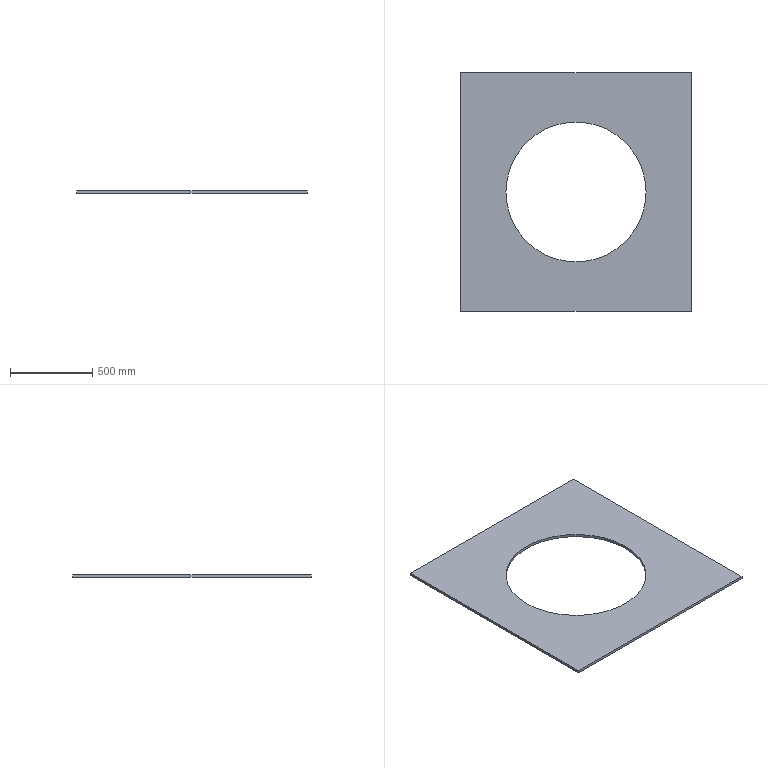Part | SolidWorks | features FlatPattern 1, ICE 1, SMBaseFlange 1, SheetMetal 1 | 1 solid | 8 faces | box 1400 x 1450 x 16 mm | volume 23400797 mm3 | plane 6 | cylinder 2 | commonest cylinder face diameters 850 x2
STEP:
#1=CARTESIAN_POINT('',(-425.,0.,-16.));
#2=VERTEX_POINT('',#1);
#3=CARTESIAN_POINT('',(425.,0.,-16.));
#4=VERTEX_POINT('',#3);
#5=CARTESIAN_POINT('',(0.,0.,-16.));
#6=DIRECTION('',(0.,0.,1.));
#7=DIRECTION('',(1.,0.,0.));
#8=AXIS2_PLACEMENT_3D('',#5,#6,#7);
#9=CIRCLE('',#8,425.);
#10=EDGE_CURVE('',#2,#4,#9,.T.);
#11=ORIENTED_EDGE('',*,*,#10,.F.);
#12=CARTESIAN_POINT('',(-425.,0.,0.));
#13=VERTEX_POINT('',#12);
#14=CARTESIAN_POINT('',(-425.,0.,-16.));
#15=DIRECTION('',(0.,0.,1.));
#16=VECTOR('',#15,1000.);
#17=LINE('',#14,#16);
#18=EDGE_CURVE('',#2,#13,#17,.T.);
#19=ORIENTED_EDGE('',*,*,#18,.T.);
#20=CARTESIAN_POINT('',(425.,0.,0.));
#21=VERTEX_POINT('',#20);
#22=CARTESIAN_POINT('',(0.,0.,0.));
#23=DIRECTION('',(0.,0.,1.));
#24=DIRECTION('',(1.,0.,0.));
#25=AXIS2_PLACEMENT_3D('',#22,#23,#24);
#26=CIRCLE('',#25,425.);
#27=EDGE_CURVE('',#13,#21,#26,.T.);
#28=ORIENTED_EDGE('',*,*,#27,.T.);
#29=CARTESIAN_POINT('',(425.,0.,-16.));
#30=DIRECTION('',(0.,0.,1.));
#31=VECTOR('',#30,1000.);
#32=LINE('',#29,#31);
#33=EDGE_CURVE('',#4,#21,#32,.T.);
#34=ORIENTED_EDGE('',*,*,#33,.F.);
#35=EDGE_LOOP('',(#11,#19,#28,#34));
#36=FACE_OUTER_BOUND('',#35,.T.);
#37=CARTESIAN_POINT('',(0.,0.,-16.));
#38=DIRECTION('',(0.,0.,1.));
#39=DIRECTION('',(1.,0.,0.));
#40=AXIS2_PLACEMENT_3D('',#37,#38,#39);
#41=CYLINDRICAL_SURFACE('',#40,425.);
#42=ADVANCED_FACE('',(#36),#41,.F.);
#43=CARTESIAN_POINT('',(700.,-725.,0.));
#44=VERTEX_POINT('',#43);
#45=CARTESIAN_POINT('',(700.,725.,0.));
#46=VERTEX_POINT('',#45);
#47=CARTESIAN_POINT('',(700.,-725.,0.));
#48=DIRECTION('',(0.,1.,0.));
#49=VECTOR('',#48,1000.);
#50=LINE('',#47,#49);
#51=EDGE_CURVE('',#44,#46,#50,.T.);
#52=ORIENTED_EDGE('',*,*,#51,.F.);
#53=CARTESIAN_POINT('',(700.,-725.,-16.));
#54=VERTEX_POINT('',#53);
#55=CARTESIAN_POINT('',(700.,-725.,-16.));
#56=DIRECTION('',(0.,0.,1.));
#57=VECTOR('',#56,1000.);
#58=LINE('',#55,#57);
#59=EDGE_CURVE('',#54,#44,#58,.T.);
#60=ORIENTED_EDGE('',*,*,#59,.F.);
#61=CARTESIAN_POINT('',(700.,725.,-16.));
#62=VERTEX_POINT('',#61);
#63=CARTESIAN_POINT('',(700.,-725.,-16.));
#64=DIRECTION('',(0.,1.,0.));
#65=VECTOR('',#64,1000.);
#66=LINE('',#63,#65);
#67=EDGE_CURVE('',#54,#62,#66,.T.);
#68=ORIENTED_EDGE('',*,*,#67,.T.);
#69=CARTESIAN_POINT('',(700.,725.,-16.));
#70=DIRECTION('',(0.,0.,1.));
#71=VECTOR('',#70,1000.);
#72=LINE('',#69,#71);
#73=EDGE_CURVE('',#62,#46,#72,.T.);
#74=ORIENTED_EDGE('',*,*,#73,.T.);
#75=EDGE_LOOP('',(#52,#60,#68,#74));
#76=FACE_OUTER_BOUND('',#75,.T.);
#77=CARTESIAN_POINT('',(700.,-725.,-16.));
#78=DIRECTION('',(1.,0.,0.));
#79=DIRECTION('',(0.,0.,-1.));
#80=AXIS2_PLACEMENT_3D('',#77,#78,#79);
#81=PLANE('',#80);
#82=ADVANCED_FACE('',(#76),#81,.T.);
#83=CARTESIAN_POINT('',(-700.,-725.,0.));
#84=VERTEX_POINT('',#83);
#85=CARTESIAN_POINT('',(-700.,-725.,0.));
#86=DIRECTION('',(1.,0.,0.));
#87=VECTOR('',#86,1000.);
#88=LINE('',#85,#87);
#89=EDGE_CURVE('',#84,#44,#88,.T.);
#90=ORIENTED_EDGE('',*,*,#89,.F.);
#91=CARTESIAN_POINT('',(-700.,-725.,-16.));
#92=VERTEX_POINT('',#91);
#93=CARTESIAN_POINT('',(-700.,-725.,-16.));
#94=DIRECTION('',(0.,0.,1.));
#95=VECTOR('',#94,1000.);
#96=LINE('',#93,#95);
#97=EDGE_CURVE('',#92,#84,#96,.T.);
#98=ORIENTED_EDGE('',*,*,#97,.F.);
#99=CARTESIAN_POINT('',(-700.,-725.,-16.));
#100=DIRECTION('',(1.,0.,0.));
#101=VECTOR('',#100,1000.);
#102=LINE('',#99,#101);
#103=EDGE_CURVE('',#92,#54,#102,.T.);
#104=ORIENTED_EDGE('',*,*,#103,.T.);
#105=ORIENTED_EDGE('',*,*,#59,.T.);
#106=EDGE_LOOP('',(#90,#98,#104,#105));
#107=FACE_OUTER_BOUND('',#106,.T.);
#108=CARTESIAN_POINT('',(-700.,-725.,-16.));
#109=DIRECTION('',(0.,-1.,0.));
#110=DIRECTION('',(0.,0.,-1.));
#111=AXIS2_PLACEMENT_3D('',#108,#109,#110);
#112=PLANE('',#111);
#113=ADVANCED_FACE('',(#107),#112,.T.);
#114=CARTESIAN_POINT('',(-700.,725.,0.));
#115=VERTEX_POINT('',#114);
#116=CARTESIAN_POINT('',(-700.,-725.,0.));
#117=DIRECTION('',(0.,-1.,0.));
#118=VECTOR('',#117,1000.);
#119=LINE('',#116,#118);
#120=EDGE_CURVE('',#115,#84,#119,.T.);
#121=ORIENTED_EDGE('',*,*,#120,.F.);
#122=CARTESIAN_POINT('',(-700.,725.,-16.));
#123=VERTEX_POINT('',#122);
#124=CARTESIAN_POINT('',(-700.,725.,-16.));
#125=DIRECTION('',(0.,0.,1.));
#126=VECTOR('',#125,1000.);
#127=LINE('',#124,#126);
#128=EDGE_CURVE('',#123,#115,#127,.T.);
#129=ORIENTED_EDGE('',*,*,#128,.F.);
#130=CARTESIAN_POINT('',(-700.,-725.,-16.));
#131=DIRECTION('',(0.,-1.,0.));
#132=VECTOR('',#131,1000.);
#133=LINE('',#130,#132);
#134=EDGE_CURVE('',#123,#92,#133,.T.);
#135=ORIENTED_EDGE('',*,*,#134,.T.);
#136=ORIENTED_EDGE('',*,*,#97,.T.);
#137=EDGE_LOOP('',(#121,#129,#135,#136));
#138=FACE_OUTER_BOUND('',#137,.T.);
#139=CARTESIAN_POINT('',(-700.,-725.,-16.));
#140=DIRECTION('',(-1.,0.,0.));
#141=DIRECTION('',(0.,0.,1.));
#142=AXIS2_PLACEMENT_3D('',#139,#140,#141);
#143=PLANE('',#142);
#144=ADVANCED_FACE('',(#138),#143,.T.);
#145=CARTESIAN_POINT('',(-700.,725.,0.));
#146=DIRECTION('',(-1.,0.,0.));
#147=VECTOR('',#146,1000.);
#148=LINE('',#145,#147);
#149=EDGE_CURVE('',#46,#115,#148,.T.);
#150=ORIENTED_EDGE('',*,*,#149,.F.);
#151=ORIENTED_EDGE('',*,*,#73,.F.);
#152=CARTESIAN_POINT('',(-700.,725.,-16.));
#153=DIRECTION('',(-1.,0.,0.));
#154=VECTOR('',#153,1000.);
#155=LINE('',#152,#154);
#156=EDGE_CURVE('',#62,#123,#155,.T.);
#157=ORIENTED_EDGE('',*,*,#156,.T.);
#158=ORIENTED_EDGE('',*,*,#128,.T.);
#159=EDGE_LOOP('',(#150,#151,#157,#158));
#160=FACE_OUTER_BOUND('',#159,.T.);
#161=CARTESIAN_POINT('',(-700.,725.,-16.));
#162=DIRECTION('',(0.,1.,0.));
#163=DIRECTION('',(0.,0.,1.));
#164=AXIS2_PLACEMENT_3D('',#161,#162,#163);
#165=PLANE('',#164);
#166=ADVANCED_FACE('',(#160),#165,.T.);
#167=CARTESIAN_POINT('',(0.,0.,-16.));
#168=DIRECTION('',(0.,0.,1.));
#169=DIRECTION('',(1.,0.,0.));
#170=AXIS2_PLACEMENT_3D('',#167,#168,#169);
#171=CIRCLE('',#170,425.);
#172=EDGE_CURVE('',#4,#2,#171,.T.);
#173=ORIENTED_EDGE('',*,*,#172,.T.);
#174=ORIENTED_EDGE('',*,*,#10,.T.);
#175=EDGE_LOOP('',(#173,#174));
#176=FACE_BOUND('',#175,.T.);
#177=ORIENTED_EDGE('',*,*,#67,.F.);
#178=ORIENTED_EDGE('',*,*,#103,.F.);
#179=ORIENTED_EDGE('',*,*,#134,.F.);
#180=ORIENTED_EDGE('',*,*,#156,.F.);
#181=EDGE_LOOP('',(#177,#178,#179,#180));
#182=FACE_OUTER_BOUND('',#181,.T.);
#183=CARTESIAN_POINT('',(0.,0.,-16.));
#184=DIRECTION('',(0.,0.,-1.));
#185=DIRECTION('',(-1.,0.,0.));
#186=AXIS2_PLACEMENT_3D('',#183,#184,#185);
#187=PLANE('',#186);
#188=ADVANCED_FACE('',(#176,#182),#187,.T.);
#189=CARTESIAN_POINT('',(0.,0.,0.));
#190=DIRECTION('',(0.,0.,1.));
#191=DIRECTION('',(1.,0.,0.));
#192=AXIS2_PLACEMENT_3D('',#189,#190,#191);
#193=CIRCLE('',#192,425.);
#194=EDGE_CURVE('',#21,#13,#193,.T.);
#195=ORIENTED_EDGE('',*,*,#194,.F.);
#196=ORIENTED_EDGE('',*,*,#27,.F.);
#197=EDGE_LOOP('',(#195,#196));
#198=FACE_BOUND('',#197,.T.);
#199=ORIENTED_EDGE('',*,*,#51,.T.);
#200=ORIENTED_EDGE('',*,*,#149,.T.);
#201=ORIENTED_EDGE('',*,*,#120,.T.);
#202=ORIENTED_EDGE('',*,*,#89,.T.);
#203=EDGE_LOOP('',(#199,#200,#201,#202));
#204=FACE_OUTER_BOUND('',#203,.T.);
#205=CARTESIAN_POINT('',(0.,0.,0.));
#206=DIRECTION('',(0.,0.,-1.));
#207=DIRECTION('',(-1.,0.,0.));
#208=AXIS2_PLACEMENT_3D('',#205,#206,#207);
#209=PLANE('',#208);
#210=ADVANCED_FACE('',(#198,#204),#209,.F.);
#211=ORIENTED_EDGE('',*,*,#18,.F.);
#212=ORIENTED_EDGE('',*,*,#172,.F.);
#213=ORIENTED_EDGE('',*,*,#33,.T.);
#214=ORIENTED_EDGE('',*,*,#194,.T.);
#215=EDGE_LOOP('',(#211,#212,#213,#214));
#216=FACE_OUTER_BOUND('',#215,.T.);
#217=CARTESIAN_POINT('',(0.,0.,-16.));
#218=DIRECTION('',(0.,0.,1.));
#219=DIRECTION('',(1.,0.,0.));
#220=AXIS2_PLACEMENT_3D('',#217,#218,#219);
#221=CYLINDRICAL_SURFACE('',#220,425.);
#222=ADVANCED_FACE('',(#216),#221,.F.);
#223=CLOSED_SHELL('',(#42,#82,#113,#144,#166,#188,#210,#222));
#224=MANIFOLD_SOLID_BREP('',#223);
#225=CARTESIAN_POINT('',(0.,0.,0.));
#226=DIRECTION('',(0.,0.,1.));
#227=DIRECTION('',(1.,0.,0.));
#228=AXIS2_PLACEMENT_3D('',#225,#226,#227);
#229=(LENGTH_UNIT()NAMED_UNIT(*)SI_UNIT(.MILLI.,.METRE.));
#230=UNCERTAINTY_MEASURE_WITH_UNIT(LENGTH_MEASURE(0.00001),#229,'','');
#231=(NAMED_UNIT(*)PLANE_ANGLE_UNIT()SI_UNIT($,.RADIAN.));
#232=(NAMED_UNIT(*)SI_UNIT($,.STERADIAN.)SOLID_ANGLE_UNIT());
#233=(GEOMETRIC_REPRESENTATION_CONTEXT(3)GLOBAL_UNCERTAINTY_ASSIGNED_CONTEXT((#230))GLOBAL_UNIT_ASSIGNED_CONTEXT((#229,#231,#232))REPRESENTATION_CONTEXT('',''));
#234=ADVANCED_BREP_SHAPE_REPRESENTATION('',(#224,#228),#233);